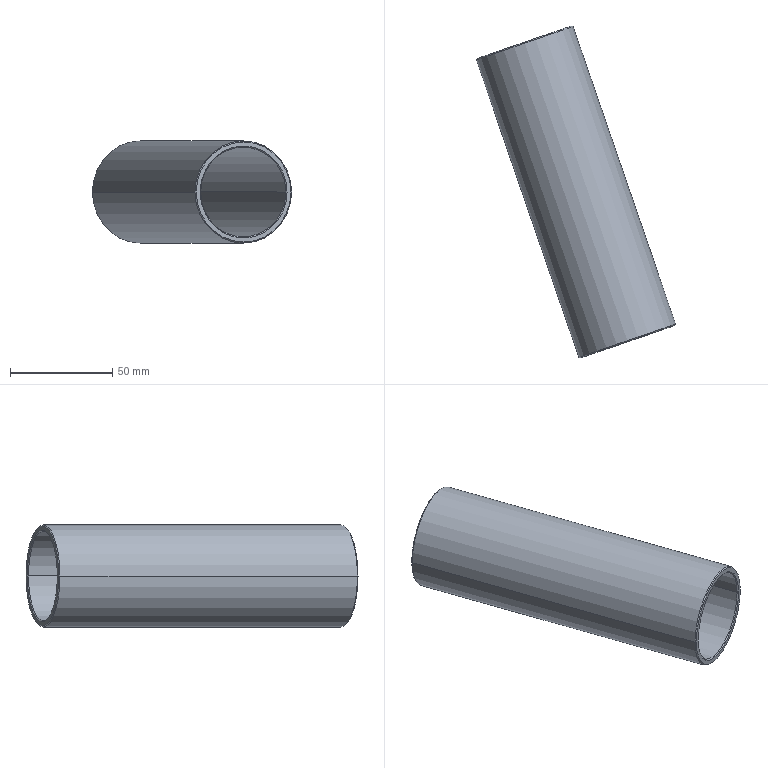Part | STEP file | PRT0001_68_1 | 1 solid | 14 faces | box 97.464 x 162.507 x 50 mm | volume 68590 mm3 | cone 8 | cylinder 4 | plane 2 | commonest cylinder face diameters 44 x2 50 x2
STEP:
#1=CARTESIAN_POINT('',(0.,0.,0.));
#2=DIRECTION('',(0.,0.,1.));
#3=DIRECTION('',(1.,0.,0.));
#4=AXIS2_PLACEMENT_3D('',#1,#2,#3);
#5=CARTESIAN_POINT('',(2166.559,1217.903,0.));
#6=VERTEX_POINT('',#5);
#7=CARTESIAN_POINT('',(2145.761,1210.732,22.));
#8=VERTEX_POINT('',#7);
#9=CARTESIAN_POINT('',(2145.761,1210.732,0.));
#10=DIRECTION('',(0.3259,-0.9454,0.));
#11=DIRECTION('',(0.9454,0.3259,0.));
#12=AXIS2_PLACEMENT_3D('',#9,#10,#11);
#13=CIRCLE('',#12,22.);
#14=CARTESIAN_POINT('',(2145.842,1210.496,0.));
#15=DIRECTION('',(0.3259,-0.9454,0.));
#16=DIRECTION('',(0.,0.,-1.));
#17=AXIS2_PLACEMENT_3D('',#14,#15,#16);
#18=CONICAL_SURFACE('',#17,22.25,0.7854);
#19=CARTESIAN_POINT('',(1.571,-0.25));
#20=DIRECTION('',(1.,0.));
#21=VECTOR('',#20,1.);
#22=LINE('',#19,#21);
#23=(GEOMETRIC_REPRESENTATION_CONTEXT(2)PARAMETRIC_REPRESENTATION_CONTEXT()REPRESENTATION_CONTEXT('',''));
#24=DEFINITIONAL_REPRESENTATION('',(#22),#23);
#25=PCURVE('',#18,#24);
#26=CARTESIAN_POINT('',(2092.545,1365.083,0.));
#27=DIRECTION('',(0.3259,-0.9454,0.));
#28=DIRECTION('',(-0.9454,-0.3259,0.));
#29=AXIS2_PLACEMENT_3D('',#26,#27,#28);
#30=CYLINDRICAL_SURFACE('',#29,22.);
#31=CARTESIAN_POINT('',(3.142,163.267));
#32=DIRECTION('',(1.,0.));
#33=VECTOR('',#32,1.);
#34=LINE('',#31,#33);
#35=(GEOMETRIC_REPRESENTATION_CONTEXT(2)PARAMETRIC_REPRESENTATION_CONTEXT()REPRESENTATION_CONTEXT('',''));
#36=DEFINITIONAL_REPRESENTATION('',(#34),#35);
#37=PCURVE('',#30,#36);
#38=SURFACE_CURVE('',#13,(#25,#37),.PCURVE_S1.);
#39=EDGE_CURVE('',#6,#8,#38,.T.);
#40=ORIENTED_EDGE('',*,*,#39,.T.);
#41=CARTESIAN_POINT('',(2124.962,1203.562,0.));
#42=VERTEX_POINT('',#41);
#43=CARTESIAN_POINT('',(2145.761,1210.732,0.));
#44=DIRECTION('',(0.3259,-0.9454,0.));
#45=DIRECTION('',(0.,0.,1.));
#46=AXIS2_PLACEMENT_3D('',#43,#44,#45);
#47=CIRCLE('',#46,22.);
#48=CARTESIAN_POINT('',(3.142,-0.25));
#49=DIRECTION('',(1.,0.));
#50=VECTOR('',#49,1.);
#51=LINE('',#48,#50);
#52=(GEOMETRIC_REPRESENTATION_CONTEXT(2)PARAMETRIC_REPRESENTATION_CONTEXT()REPRESENTATION_CONTEXT('',''));
#53=DEFINITIONAL_REPRESENTATION('',(#51),#52);
#54=PCURVE('',#18,#53);
#55=CARTESIAN_POINT('',(4.712,163.267));
#56=DIRECTION('',(1.,0.));
#57=VECTOR('',#56,1.);
#58=LINE('',#55,#57);
#59=(GEOMETRIC_REPRESENTATION_CONTEXT(2)PARAMETRIC_REPRESENTATION_CONTEXT()REPRESENTATION_CONTEXT('',''));
#60=DEFINITIONAL_REPRESENTATION('',(#58),#59);
#61=PCURVE('',#30,#60);
#62=SURFACE_CURVE('',#47,(#54,#61),.PCURVE_S1.);
#63=EDGE_CURVE('',#8,#42,#62,.T.);
#64=ORIENTED_EDGE('',*,*,#63,.T.);
#65=CARTESIAN_POINT('',(2124.653,1202.926,0.));
#66=VERTEX_POINT('',#65);
#67=CARTESIAN_POINT('',(2124.653,1202.926,0.));
#68=DIRECTION('',(0.438,0.899,0.));
#69=VECTOR('',#68,1.);
#70=LINE('',#67,#69);
#71=CARTESIAN_POINT('',(4.712,0.25));
#72=DIRECTION('',(0.,-1.));
#73=VECTOR('',#72,1.);
#74=LINE('',#71,#73);
#75=(GEOMETRIC_REPRESENTATION_CONTEXT(2)PARAMETRIC_REPRESENTATION_CONTEXT()REPRESENTATION_CONTEXT('',''));
#76=DEFINITIONAL_REPRESENTATION('',(#74),#75);
#77=PCURVE('',#18,#76);
#78=CARTESIAN_POINT('',(2145.842,1210.496,0.));
#79=DIRECTION('',(0.3259,-0.9454,0.));
#80=DIRECTION('',(0.,0.,-1.));
#81=AXIS2_PLACEMENT_3D('',#78,#79,#80);
#82=CONICAL_SURFACE('',#81,22.25,0.7854);
#83=CARTESIAN_POINT('',(4.712,0.25));
#84=DIRECTION('',(0.,-1.));
#85=VECTOR('',#84,1.);
#86=LINE('',#83,#85);
#87=(GEOMETRIC_REPRESENTATION_CONTEXT(2)PARAMETRIC_REPRESENTATION_CONTEXT()REPRESENTATION_CONTEXT('',''));
#88=DEFINITIONAL_REPRESENTATION('',(#86),#87);
#89=PCURVE('',#82,#88);
#90=SURFACE_CURVE('',#70,(#77,#89),.PCURVE_S1.);
#91=EDGE_CURVE('',#66,#42,#90,.T.);
#92=ORIENTED_EDGE('',*,*,#91,.F.);
#93=CARTESIAN_POINT('',(2145.924,1210.26,22.5));
#94=VERTEX_POINT('',#93);
#95=CARTESIAN_POINT('',(2145.924,1210.26,0.));
#96=DIRECTION('',(0.3259,-0.9454,0.));
#97=DIRECTION('',(0.,0.,1.));
#98=AXIS2_PLACEMENT_3D('',#95,#96,#97);
#99=CIRCLE('',#98,22.5);
#100=CARTESIAN_POINT('',(3.142,0.25));
#101=DIRECTION('',(1.,0.));
#102=VECTOR('',#101,1.);
#103=LINE('',#100,#102);
#104=(GEOMETRIC_REPRESENTATION_CONTEXT(2)PARAMETRIC_REPRESENTATION_CONTEXT()REPRESENTATION_CONTEXT('',''));
#105=DEFINITIONAL_REPRESENTATION('',(#103),#104);
#106=PCURVE('',#18,#105);
#107=CARTESIAN_POINT('',(2145.924,1210.26,0.));
#108=DIRECTION('',(0.3259,-0.9454,0.));
#109=DIRECTION('',(-0.9454,-0.3259,0.));
#110=AXIS2_PLACEMENT_3D('',#107,#108,#109);
#111=PLANE('',#110);
#112=CARTESIAN_POINT('',(-0.000000001,0.));
#113=DIRECTION('',(0.,-1.));
#114=AXIS2_PLACEMENT_2D('',#112,#113);
#115=CIRCLE('',#114,22.5);
#116=(GEOMETRIC_REPRESENTATION_CONTEXT(2)PARAMETRIC_REPRESENTATION_CONTEXT()REPRESENTATION_CONTEXT('',''));
#117=DEFINITIONAL_REPRESENTATION('',(#115),#116);
#118=PCURVE('',#111,#117);
#119=SURFACE_CURVE('',#99,(#106,#118),.PCURVE_S1.);
#120=EDGE_CURVE('',#94,#66,#119,.T.);
#121=ORIENTED_EDGE('',*,*,#120,.F.);
#122=CARTESIAN_POINT('',(2167.195,1217.593,0.));
#123=VERTEX_POINT('',#122);
#124=CARTESIAN_POINT('',(2145.924,1210.26,0.));
#125=DIRECTION('',(0.3259,-0.9454,0.));
#126=DIRECTION('',(0.9454,0.3259,0.));
#127=AXIS2_PLACEMENT_3D('',#124,#125,#126);
#128=CIRCLE('',#127,22.5);
#129=CARTESIAN_POINT('',(1.571,0.25));
#130=DIRECTION('',(1.,0.));
#131=VECTOR('',#130,1.);
#132=LINE('',#129,#131);
#133=(GEOMETRIC_REPRESENTATION_CONTEXT(2)PARAMETRIC_REPRESENTATION_CONTEXT()REPRESENTATION_CONTEXT('',''));
#134=DEFINITIONAL_REPRESENTATION('',(#132),#133);
#135=PCURVE('',#18,#134);
#136=CARTESIAN_POINT('',(-0.000000001,0.));
#137=DIRECTION('',(-1.,0.));
#138=AXIS2_PLACEMENT_2D('',#136,#137);
#139=CIRCLE('',#138,22.5);
#140=(GEOMETRIC_REPRESENTATION_CONTEXT(2)PARAMETRIC_REPRESENTATION_CONTEXT()REPRESENTATION_CONTEXT('',''));
#141=DEFINITIONAL_REPRESENTATION('',(#139),#140);
#142=PCURVE('',#111,#141);
#143=SURFACE_CURVE('',#128,(#135,#142),.PCURVE_S1.);
#144=EDGE_CURVE('',#123,#94,#143,.T.);
#145=ORIENTED_EDGE('',*,*,#144,.F.);
#146=CARTESIAN_POINT('',(2167.195,1217.593,0.));
#147=DIRECTION('',(-0.899,0.438,0.));
#148=VECTOR('',#147,1.);
#149=LINE('',#146,#148);
#150=CARTESIAN_POINT('',(1.571,0.25));
#151=DIRECTION('',(0.,-1.));
#152=VECTOR('',#151,1.);
#153=LINE('',#150,#152);
#154=(GEOMETRIC_REPRESENTATION_CONTEXT(2)PARAMETRIC_REPRESENTATION_CONTEXT()REPRESENTATION_CONTEXT('',''));
#155=DEFINITIONAL_REPRESENTATION('',(#153),#154);
#156=PCURVE('',#18,#155);
#157=CARTESIAN_POINT('',(7.854,0.25));
#158=DIRECTION('',(0.,-1.));
#159=VECTOR('',#158,1.);
#160=LINE('',#157,#159);
#161=(GEOMETRIC_REPRESENTATION_CONTEXT(2)PARAMETRIC_REPRESENTATION_CONTEXT()REPRESENTATION_CONTEXT('',''));
#162=DEFINITIONAL_REPRESENTATION('',(#160),#161);
#163=PCURVE('',#82,#162);
#164=SURFACE_CURVE('',#149,(#156,#163),.PCURVE_S1.);
#165=EDGE_CURVE('',#123,#6,#164,.T.);
#166=ORIENTED_EDGE('',*,*,#165,.T.);
#167=EDGE_LOOP('',(#40,#64,#92,#121,#145,#166));
#168=FACE_BOUND('',#167,.F.);
#169=ADVANCED_FACE('',(#168),#18,.F.);
#170=CARTESIAN_POINT('',(2095.566,1356.322,22.));
#171=VERTEX_POINT('',#170);
#172=CARTESIAN_POINT('',(2116.364,1363.493,0.));
#173=VERTEX_POINT('',#172);
#174=CARTESIAN_POINT('',(2095.566,1356.322,0.));
#175=DIRECTION('',(-0.3259,0.9454,0.));
#176=DIRECTION('',(0.,0.,1.));
#177=AXIS2_PLACEMENT_3D('',#174,#175,#176);
#178=CIRCLE('',#177,22.);
#179=CARTESIAN_POINT('',(4.712,9.267));
#180=DIRECTION('',(-1.,0.));
#181=VECTOR('',#180,1.);
#182=LINE('',#179,#181);
#183=(GEOMETRIC_REPRESENTATION_CONTEXT(2)PARAMETRIC_REPRESENTATION_CONTEXT()REPRESENTATION_CONTEXT('',''));
#184=DEFINITIONAL_REPRESENTATION('',(#182),#183);
#185=PCURVE('',#30,#184);
#186=CARTESIAN_POINT('',(2095.484,1356.559,0.));
#187=DIRECTION('',(-0.3259,0.9454,0.));
#188=DIRECTION('',(0.,0.,-1.));
#189=AXIS2_PLACEMENT_3D('',#186,#187,#188);
#190=CONICAL_SURFACE('',#189,22.25,0.7854);
#191=CARTESIAN_POINT('',(3.142,-0.25));
#192=DIRECTION('',(1.,0.));
#193=VECTOR('',#192,1.);
#194=LINE('',#191,#193);
#195=(GEOMETRIC_REPRESENTATION_CONTEXT(2)PARAMETRIC_REPRESENTATION_CONTEXT()REPRESENTATION_CONTEXT('',''));
#196=DEFINITIONAL_REPRESENTATION('',(#194),#195);
#197=PCURVE('',#190,#196);
#198=SURFACE_CURVE('',#178,(#185,#197),.PCURVE_S1.);
#199=EDGE_CURVE('',#171,#173,#198,.T.);
#200=ORIENTED_EDGE('',*,*,#199,.F.);
#201=CARTESIAN_POINT('',(2074.767,1349.152,0.));
#202=VERTEX_POINT('',#201);
#203=CARTESIAN_POINT('',(2095.566,1356.322,0.));
#204=DIRECTION('',(-0.3259,0.9454,0.));
#205=DIRECTION('',(-0.9454,-0.3259,0.));
#206=AXIS2_PLACEMENT_3D('',#203,#204,#205);
#207=CIRCLE('',#206,22.);
#208=CARTESIAN_POINT('',(6.283,9.267));
#209=DIRECTION('',(-1.,0.));
#210=VECTOR('',#209,1.);
#211=LINE('',#208,#210);
#212=(GEOMETRIC_REPRESENTATION_CONTEXT(2)PARAMETRIC_REPRESENTATION_CONTEXT()REPRESENTATION_CONTEXT('',''));
#213=DEFINITIONAL_REPRESENTATION('',(#211),#212);
#214=PCURVE('',#30,#213);
#215=CARTESIAN_POINT('',(1.571,-0.25));
#216=DIRECTION('',(1.,0.));
#217=VECTOR('',#216,1.);
#218=LINE('',#215,#217);
#219=(GEOMETRIC_REPRESENTATION_CONTEXT(2)PARAMETRIC_REPRESENTATION_CONTEXT()REPRESENTATION_CONTEXT('',''));
#220=DEFINITIONAL_REPRESENTATION('',(#218),#219);
#221=PCURVE('',#190,#220);
#222=SURFACE_CURVE('',#207,(#214,#221),.PCURVE_S1.);
#223=EDGE_CURVE('',#202,#171,#222,.T.);
#224=ORIENTED_EDGE('',*,*,#223,.F.);
#225=CARTESIAN_POINT('',(2074.767,1349.152,0.));
#226=DIRECTION('',(0.3259,-0.9454,0.));
#227=VECTOR('',#226,1.);
#228=LINE('',#225,#227);
#229=CARTESIAN_POINT('',(6.283,9.267));
#230=DIRECTION('',(0.,1.));
#231=VECTOR('',#230,1.);
#232=LINE('',#229,#231);
#233=(GEOMETRIC_REPRESENTATION_CONTEXT(2)PARAMETRIC_REPRESENTATION_CONTEXT()REPRESENTATION_CONTEXT('',''));
#234=DEFINITIONAL_REPRESENTATION('',(#232),#233);
#235=PCURVE('',#30,#234);
#236=CARTESIAN_POINT('',(2092.545,1365.083,0.));
#237=DIRECTION('',(0.3259,-0.9454,0.));
#238=DIRECTION('',(-0.9454,-0.3259,0.));
#239=AXIS2_PLACEMENT_3D('',#236,#237,#238);
#240=CYLINDRICAL_SURFACE('',#239,22.);
#241=CARTESIAN_POINT('',(0.,9.267));
#242=DIRECTION('',(0.,1.));
#243=VECTOR('',#242,1.);
#244=LINE('',#241,#243);
#245=(GEOMETRIC_REPRESENTATION_CONTEXT(2)PARAMETRIC_REPRESENTATION_CONTEXT()REPRESENTATION_CONTEXT('',''));
#246=DEFINITIONAL_REPRESENTATION('',(#244),#245);
#247=PCURVE('',#240,#246);
#248=SURFACE_CURVE('',#228,(#235,#247),.PCURVE_S1.);
#249=EDGE_CURVE('',#202,#42,#248,.T.);
#250=ORIENTED_EDGE('',*,*,#249,.T.);
#251=ORIENTED_EDGE('',*,*,#63,.F.);
#252=ORIENTED_EDGE('',*,*,#39,.F.);
#253=CARTESIAN_POINT('',(2116.364,1363.493,0.));
#254=DIRECTION('',(0.3259,-0.9454,0.));
#255=VECTOR('',#254,1.);
#256=LINE('',#253,#255);
#257=CARTESIAN_POINT('',(3.142,9.267));
#258=DIRECTION('',(0.,1.));
#259=VECTOR('',#258,1.);
#260=LINE('',#257,#259);
#261=(GEOMETRIC_REPRESENTATION_CONTEXT(2)PARAMETRIC_REPRESENTATION_CONTEXT()REPRESENTATION_CONTEXT('',''));
#262=DEFINITIONAL_REPRESENTATION('',(#260),#261);
#263=PCURVE('',#30,#262);
#264=CARTESIAN_POINT('',(3.142,9.267));
#265=DIRECTION('',(0.,1.));
#266=VECTOR('',#265,1.);
#267=LINE('',#264,#266);
#268=(GEOMETRIC_REPRESENTATION_CONTEXT(2)PARAMETRIC_REPRESENTATION_CONTEXT()REPRESENTATION_CONTEXT('',''));
#269=DEFINITIONAL_REPRESENTATION('',(#267),#268);
#270=PCURVE('',#240,#269);
#271=SURFACE_CURVE('',#256,(#263,#270),.PCURVE_S1.);
#272=EDGE_CURVE('',#173,#6,#271,.T.);
#273=ORIENTED_EDGE('',*,*,#272,.F.);
#274=EDGE_LOOP('',(#200,#224,#250,#251,#252,#273));
#275=FACE_BOUND('',#274,.F.);
#276=ADVANCED_FACE('',(#275),#30,.F.);
#277=CARTESIAN_POINT('',(2095.403,1356.795,22.5));
#278=VERTEX_POINT('',#277);
#279=CARTESIAN_POINT('',(2116.674,1364.129,0.));
#280=VERTEX_POINT('',#279);
#281=CARTESIAN_POINT('',(2095.403,1356.795,0.));
#282=DIRECTION('',(-0.3259,0.9454,0.));
#283=DIRECTION('',(0.,0.,1.));
#284=AXIS2_PLACEMENT_3D('',#281,#282,#283);
#285=CIRCLE('',#284,22.5);
#286=CARTESIAN_POINT('',(3.142,0.25));
#287=DIRECTION('',(1.,0.));
#288=VECTOR('',#287,1.);
#289=LINE('',#286,#288);
#290=(GEOMETRIC_REPRESENTATION_CONTEXT(2)PARAMETRIC_REPRESENTATION_CONTEXT()REPRESENTATION_CONTEXT('',''));
#291=DEFINITIONAL_REPRESENTATION('',(#289),#290);
#292=PCURVE('',#190,#291);
#293=CARTESIAN_POINT('',(2095.403,1356.795,0.));
#294=DIRECTION('',(0.3259,-0.9454,0.));
#295=DIRECTION('',(-0.9454,-0.3259,0.));
#296=AXIS2_PLACEMENT_3D('',#293,#294,#295);
#297=PLANE('',#296);
#298=CARTESIAN_POINT('',(0.,-22.5));
#299=CARTESIAN_POINT('',(-38.971,-22.5));
#300=CARTESIAN_POINT('',(-19.485,11.25));
#301=CARTESIAN_POINT('',(0.,45.));
#302=CARTESIAN_POINT('',(19.485,11.25));
#303=CARTESIAN_POINT('',(38.971,-22.5));
#304=CARTESIAN_POINT('',(0.,-22.5));
#305=(BOUNDED_CURVE()B_SPLINE_CURVE(2,(#298,#299,#300,#301,#302,#303,#304),.UNSPECIFIED.,.T.,.F.)B_SPLINE_CURVE_WITH_KNOTS((1,2,2,2,2,1),(-2.094,0.,2.094,4.189,6.283,8.378),.UNSPECIFIED.)CURVE()GEOMETRIC_REPRESENTATION_ITEM()RATIONAL_B_SPLINE_CURVE((1.,0.5,1.,0.5,1.,0.5,1.))REPRESENTATION_ITEM(''));
#306=(GEOMETRIC_REPRESENTATION_CONTEXT(2)PARAMETRIC_REPRESENTATION_CONTEXT()REPRESENTATION_CONTEXT('',''));
#307=DEFINITIONAL_REPRESENTATION('',(#305),#306);
#308=PCURVE('',#297,#307);
#309=SURFACE_CURVE('',#285,(#292,#308),.PCURVE_S1.);
#310=EDGE_CURVE('',#278,#280,#309,.T.);
#311=ORIENTED_EDGE('',*,*,#310,.F.);
#312=CARTESIAN_POINT('',(2074.132,1349.461,0.));
#313=VERTEX_POINT('',#312);
#314=CARTESIAN_POINT('',(2095.403,1356.795,0.));
#315=DIRECTION('',(-0.3259,0.9454,0.));
#316=DIRECTION('',(-0.9454,-0.3259,0.));
#317=AXIS2_PLACEMENT_3D('',#314,#315,#316);
#318=CIRCLE('',#317,22.5);
#319=CARTESIAN_POINT('',(1.571,0.25));
#320=DIRECTION('',(1.,0.));
#321=VECTOR('',#320,1.);
#322=LINE('',#319,#321);
#323=(GEOMETRIC_REPRESENTATION_CONTEXT(2)PARAMETRIC_REPRESENTATION_CONTEXT()REPRESENTATION_CONTEXT('',''));
#324=DEFINITIONAL_REPRESENTATION('',(#322),#323);
#325=PCURVE('',#190,#324);
#326=CARTESIAN_POINT('',(22.5,0.));
#327=CARTESIAN_POINT('',(22.5,-38.971));
#328=CARTESIAN_POINT('',(-11.25,-19.485));
#329=CARTESIAN_POINT('',(-45.,0.));
#330=CARTESIAN_POINT('',(-11.25,19.485));
#331=CARTESIAN_POINT('',(22.5,38.971));
#332=CARTESIAN_POINT('',(22.5,0.));
#333=(BOUNDED_CURVE()B_SPLINE_CURVE(2,(#326,#327,#328,#329,#330,#331,#332),.UNSPECIFIED.,.T.,.F.)B_SPLINE_CURVE_WITH_KNOTS((1,2,2,2,2,1),(-2.094,0.,2.094,4.189,6.283,8.378),.UNSPECIFIED.)CURVE()GEOMETRIC_REPRESENTATION_ITEM()RATIONAL_B_SPLINE_CURVE((1.,0.5,1.,0.5,1.,0.5,1.))REPRESENTATION_ITEM(''));
#334=(GEOMETRIC_REPRESENTATION_CONTEXT(2)PARAMETRIC_REPRESENTATION_CONTEXT()REPRESENTATION_CONTEXT('',''));
#335=DEFINITIONAL_REPRESENTATION('',(#333),#334);
#336=PCURVE('',#297,#335);
#337=SURFACE_CURVE('',#318,(#325,#336),.PCURVE_S1.);
#338=EDGE_CURVE('',#313,#278,#337,.T.);
#339=ORIENTED_EDGE('',*,*,#338,.F.);
#340=CARTESIAN_POINT('',(2074.767,1349.152,0.));
#341=DIRECTION('',(-0.899,0.438,0.));
#342=VECTOR('',#341,1.);
#343=LINE('',#340,#342);
#344=CARTESIAN_POINT('',(1.571,-0.25));
#345=DIRECTION('',(0.,1.));
#346=VECTOR('',#345,1.);
#347=LINE('',#344,#346);
#348=(GEOMETRIC_REPRESENTATION_CONTEXT(2)PARAMETRIC_REPRESENTATION_CONTEXT()REPRESENTATION_CONTEXT('',''));
#349=DEFINITIONAL_REPRESENTATION('',(#347),#348);
#350=PCURVE('',#190,#349);
#351=CARTESIAN_POINT('',(2095.484,1356.559,0.));
#352=DIRECTION('',(-0.3259,0.9454,0.));
#353=DIRECTION('',(0.,0.,-1.));
#354=AXIS2_PLACEMENT_3D('',#351,#352,#353);
#355=CONICAL_SURFACE('',#354,22.25,0.7854);
#356=CARTESIAN_POINT('',(1.571,-0.25));
#357=DIRECTION('',(0.,1.));
#358=VECTOR('',#357,1.);
#359=LINE('',#356,#358);
#360=(GEOMETRIC_REPRESENTATION_CONTEXT(2)PARAMETRIC_REPRESENTATION_CONTEXT()REPRESENTATION_CONTEXT('',''));
#361=DEFINITIONAL_REPRESENTATION('',(#359),#360);
#362=PCURVE('',#355,#361);
#363=SURFACE_CURVE('',#343,(#350,#362),.PCURVE_S1.);
#364=EDGE_CURVE('',#202,#313,#363,.T.);
#365=ORIENTED_EDGE('',*,*,#364,.F.);
#366=ORIENTED_EDGE('',*,*,#223,.T.);
#367=ORIENTED_EDGE('',*,*,#199,.T.);
#368=CARTESIAN_POINT('',(2116.364,1363.493,0.));
#369=DIRECTION('',(0.438,0.899,0.));
#370=VECTOR('',#369,1.);
#371=LINE('',#368,#370);
#372=CARTESIAN_POINT('',(4.712,-0.25));
#373=DIRECTION('',(0.,1.));
#374=VECTOR('',#373,1.);
#375=LINE('',#372,#374);
#376=(GEOMETRIC_REPRESENTATION_CONTEXT(2)PARAMETRIC_REPRESENTATION_CONTEXT()REPRESENTATION_CONTEXT('',''));
#377=DEFINITIONAL_REPRESENTATION('',(#375),#376);
#378=PCURVE('',#190,#377);
#379=CARTESIAN_POINT('',(-1.571,-0.25));
#380=DIRECTION('',(0.,1.));
#381=VECTOR('',#380,1.);
#382=LINE('',#379,#381);
#383=(GEOMETRIC_REPRESENTATION_CONTEXT(2)PARAMETRIC_REPRESENTATION_CONTEXT()REPRESENTATION_CONTEXT('',''));
#384=DEFINITIONAL_REPRESENTATION('',(#382),#383);
#385=PCURVE('',#355,#384);
#386=SURFACE_CURVE('',#371,(#378,#385),.PCURVE_S1.);
#387=EDGE_CURVE('',#173,#280,#386,.T.);
#388=ORIENTED_EDGE('',*,*,#387,.T.);
#389=EDGE_LOOP('',(#311,#339,#365,#366,#367,#388));
#390=FACE_BOUND('',#389,.F.);
#391=ADVANCED_FACE('',(#390),#190,.F.);
#392=CARTESIAN_POINT('',(2072.241,1348.809,0.));
#393=VERTEX_POINT('',#392);
#394=CARTESIAN_POINT('',(2095.403,1356.795,-24.5));
#395=VERTEX_POINT('',#394);
#396=CARTESIAN_POINT('',(2095.403,1356.795,0.));
#397=DIRECTION('',(0.3259,-0.9454,0.));
#398=DIRECTION('',(-0.9454,-0.3259,0.));
#399=AXIS2_PLACEMENT_3D('',#396,#397,#398);
#400=CIRCLE('',#399,24.5);
#401=CARTESIAN_POINT('',(0.,0.));
#402=DIRECTION('',(1.,0.));
#403=AXIS2_PLACEMENT_2D('',#401,#402);
#404=CIRCLE('',#403,24.5);
#405=(GEOMETRIC_REPRESENTATION_CONTEXT(2)PARAMETRIC_REPRESENTATION_CONTEXT()REPRESENTATION_CONTEXT('',''));
#406=DEFINITIONAL_REPRESENTATION('',(#404),#405);
#407=PCURVE('',#297,#406);
#408=CARTESIAN_POINT('',(2095.484,1356.559,0.));
#409=DIRECTION('',(0.3259,-0.9454,0.));
#410=DIRECTION('',(0.,0.,-1.));
#411=AXIS2_PLACEMENT_3D('',#408,#409,#410);
#412=CONICAL_SURFACE('',#411,24.75,0.7854);
#413=CARTESIAN_POINT('',(-1.571,-0.25));
#414=DIRECTION('',(1.,0.));
#415=VECTOR('',#414,1.);
#416=LINE('',#413,#415);
#417=(GEOMETRIC_REPRESENTATION_CONTEXT(2)PARAMETRIC_REPRESENTATION_CONTEXT()REPRESENTATION_CONTEXT('',''));
#418=DEFINITIONAL_REPRESENTATION('',(#416),#417);
#419=PCURVE('',#412,#418);
#420=SURFACE_CURVE('',#400,(#407,#419),.PCURVE_S1.);
#421=EDGE_CURVE('',#393,#395,#420,.T.);
#422=ORIENTED_EDGE('',*,*,#421,.T.);
#423=CARTESIAN_POINT('',(2118.565,1364.781,0.));
#424=VERTEX_POINT('',#423);
#425=CARTESIAN_POINT('',(2095.403,1356.795,0.));
#426=DIRECTION('',(0.3259,-0.9454,0.));
#427=DIRECTION('',(0.,0.,-1.));
#428=AXIS2_PLACEMENT_3D('',#425,#426,#427);
#429=CIRCLE('',#428,24.5);
#430=CARTESIAN_POINT('',(0.,0.));
#431=DIRECTION('',(0.,1.));
#432=AXIS2_PLACEMENT_2D('',#430,#431);
#433=CIRCLE('',#432,24.5);
#434=(GEOMETRIC_REPRESENTATION_CONTEXT(2)PARAMETRIC_REPRESENTATION_CONTEXT()REPRESENTATION_CONTEXT('',''));
#435=DEFINITIONAL_REPRESENTATION('',(#433),#434);
#436=PCURVE('',#297,#435);
#437=CARTESIAN_POINT('',(0.,-0.25));
#438=DIRECTION('',(1.,0.));
#439=VECTOR('',#438,1.);
#440=LINE('',#437,#439);
#441=(GEOMETRIC_REPRESENTATION_CONTEXT(2)PARAMETRIC_REPRESENTATION_CONTEXT()REPRESENTATION_CONTEXT('',''));
#442=DEFINITIONAL_REPRESENTATION('',(#440),#441);
#443=PCURVE('',#412,#442);
#444=SURFACE_CURVE('',#429,(#436,#443),.PCURVE_S1.);
#445=EDGE_CURVE('',#395,#424,#444,.T.);
#446=ORIENTED_EDGE('',*,*,#445,.T.);
#447=CARTESIAN_POINT('',(2095.403,1356.795,24.5));
#448=VERTEX_POINT('',#447);
#449=CARTESIAN_POINT('',(2095.403,1356.795,0.));
#450=DIRECTION('',(0.3259,-0.9454,0.));
#451=DIRECTION('',(0.9454,0.3259,0.));
#452=AXIS2_PLACEMENT_3D('',#449,#450,#451);
#453=CIRCLE('',#452,24.5);
#454=CARTESIAN_POINT('',(0.,0.));
#455=DIRECTION('',(-1.,0.));
#456=AXIS2_PLACEMENT_2D('',#454,#455);
#457=CIRCLE('',#456,24.5);
#458=(GEOMETRIC_REPRESENTATION_CONTEXT(2)PARAMETRIC_REPRESENTATION_CONTEXT()REPRESENTATION_CONTEXT('',''));
#459=DEFINITIONAL_REPRESENTATION('',(#457),#458);
#460=PCURVE('',#297,#459);
#461=CARTESIAN_POINT('',(2095.484,1356.559,0.));
#462=DIRECTION('',(0.3259,-0.9454,0.));
#463=DIRECTION('',(0.,0.,-1.));
#464=AXIS2_PLACEMENT_3D('',#461,#462,#463);
#465=CONICAL_SURFACE('',#464,24.75,0.7854);
#466=CARTESIAN_POINT('',(1.571,-0.25));
#467=DIRECTION('',(1.,0.));
#468=VECTOR('',#467,1.);
#469=LINE('',#466,#468);
#470=(GEOMETRIC_REPRESENTATION_CONTEXT(2)PARAMETRIC_REPRESENTATION_CONTEXT()REPRESENTATION_CONTEXT('',''));
#471=DEFINITIONAL_REPRESENTATION('',(#469),#470);
#472=PCURVE('',#465,#471);
#473=SURFACE_CURVE('',#453,(#460,#472),.PCURVE_S1.);
#474=EDGE_CURVE('',#424,#448,#473,.T.);
#475=ORIENTED_EDGE('',*,*,#474,.T.);
#476=CARTESIAN_POINT('',(2095.403,1356.795,0.));
#477=DIRECTION('',(0.3259,-0.9454,0.));
#478=DIRECTION('',(0.,0.,1.));
#479=AXIS2_PLACEMENT_3D('',#476,#477,#478);
#480=CIRCLE('',#479,24.5);
#481=CARTESIAN_POINT('',(0.,0.));
#482=DIRECTION('',(0.,-1.));
#483=AXIS2_PLACEMENT_2D('',#481,#482);
#484=CIRCLE('',#483,24.5);
#485=(GEOMETRIC_REPRESENTATION_CONTEXT(2)PARAMETRIC_REPRESENTATION_CONTEXT()REPRESENTATION_CONTEXT('',''));
#486=DEFINITIONAL_REPRESENTATION('',(#484),#485);
#487=PCURVE('',#297,#486);
#488=CARTESIAN_POINT('',(3.142,-0.25));
#489=DIRECTION('',(1.,0.));
#490=VECTOR('',#489,1.);
#491=LINE('',#488,#490);
#492=(GEOMETRIC_REPRESENTATION_CONTEXT(2)PARAMETRIC_REPRESENTATION_CONTEXT()REPRESENTATION_CONTEXT('',''));
#493=DEFINITIONAL_REPRESENTATION('',(#491),#492);
#494=PCURVE('',#465,#493);
#495=SURFACE_CURVE('',#480,(#487,#494),.PCURVE_S1.);
#496=EDGE_CURVE('',#448,#393,#495,.T.);
#497=ORIENTED_EDGE('',*,*,#496,.T.);
#498=EDGE_LOOP('',(#422,#446,#475,#497));
#499=FACE_BOUND('',#498,.F.);
#500=CARTESIAN_POINT('',(2095.403,1356.795,-22.5));
#501=VERTEX_POINT('',#500);
#502=CARTESIAN_POINT('',(2095.403,1356.795,0.));
#503=DIRECTION('',(-0.3259,0.9454,0.));
#504=DIRECTION('',(0.9454,0.3259,0.));
#505=AXIS2_PLACEMENT_3D('',#502,#503,#504);
#506=CIRCLE('',#505,22.5);
#507=CARTESIAN_POINT('',(-22.5,0.));
#508=CARTESIAN_POINT('',(-22.5,38.971));
#509=CARTESIAN_POINT('',(11.25,19.485));
#510=CARTESIAN_POINT('',(45.,0.));
#511=CARTESIAN_POINT('',(11.25,-19.485));
#512=CARTESIAN_POINT('',(-22.5,-38.971));
#513=CARTESIAN_POINT('',(-22.5,0.));
#514=(BOUNDED_CURVE()B_SPLINE_CURVE(2,(#507,#508,#509,#510,#511,#512,#513),.UNSPECIFIED.,.T.,.F.)B_SPLINE_CURVE_WITH_KNOTS((1,2,2,2,2,1),(-2.094,0.,2.094,4.189,6.283,8.378),.UNSPECIFIED.)CURVE()GEOMETRIC_REPRESENTATION_ITEM()RATIONAL_B_SPLINE_CURVE((1.,0.5,1.,0.5,1.,0.5,1.))REPRESENTATION_ITEM(''));
#515=(GEOMETRIC_REPRESENTATION_CONTEXT(2)PARAMETRIC_REPRESENTATION_CONTEXT()REPRESENTATION_CONTEXT('',''));
#516=DEFINITIONAL_REPRESENTATION('',(#514),#515);
#517=PCURVE('',#297,#516);
#518=CARTESIAN_POINT('',(-1.571,0.25));
#519=DIRECTION('',(1.,0.));
#520=VECTOR('',#519,1.);
#521=LINE('',#518,#520);
#522=(GEOMETRIC_REPRESENTATION_CONTEXT(2)PARAMETRIC_REPRESENTATION_CONTEXT()REPRESENTATION_CONTEXT('',''));
#523=DEFINITIONAL_REPRESENTATION('',(#521),#522);
#524=PCURVE('',#355,#523);
#525=SURFACE_CURVE('',#506,(#517,#524),.PCURVE_S1.);
#526=EDGE_CURVE('',#280,#501,#525,.T.);
#527=ORIENTED_EDGE('',*,*,#526,.T.);
#528=CARTESIAN_POINT('',(2095.403,1356.795,0.));
#529=DIRECTION('',(-0.3259,0.9454,0.));
#530=DIRECTION('',(0.,0.,-1.));
#531=AXIS2_PLACEMENT_3D('',#528,#529,#530);
#532=CIRCLE('',#531,22.5);
#533=CARTESIAN_POINT('',(0.,22.5));
#534=CARTESIAN_POINT('',(38.971,22.5));
#535=CARTESIAN_POINT('',(19.485,-11.25));
#536=CARTESIAN_POINT('',(0.,-45.));
#537=CARTESIAN_POINT('',(-19.485,-11.25));
#538=CARTESIAN_POINT('',(-38.971,22.5));
#539=CARTESIAN_POINT('',(0.,22.5));
#540=(BOUNDED_CURVE()B_SPLINE_CURVE(2,(#533,#534,#535,#536,#537,#538,#539),.UNSPECIFIED.,.T.,.F.)B_SPLINE_CURVE_WITH_KNOTS((1,2,2,2,2,1),(-2.094,0.,2.094,4.189,6.283,8.378),.UNSPECIFIED.)CURVE()GEOMETRIC_REPRESENTATION_ITEM()RATIONAL_B_SPLINE_CURVE((1.,0.5,1.,0.5,1.,0.5,1.))REPRESENTATION_ITEM(''));
#541=(GEOMETRIC_REPRESENTATION_CONTEXT(2)PARAMETRIC_REPRESENTATION_CONTEXT()REPRESENTATION_CONTEXT('',''));
#542=DEFINITIONAL_REPRESENTATION('',(#540),#541);
#543=PCURVE('',#297,#542);
#544=CARTESIAN_POINT('',(0.,0.25));
#545=DIRECTION('',(1.,0.));
#546=VECTOR('',#545,1.);
#547=LINE('',#544,#546);
#548=(GEOMETRIC_REPRESENTATION_CONTEXT(2)PARAMETRIC_REPRESENTATION_CONTEXT()REPRESENTATION_CONTEXT('',''));
#549=DEFINITIONAL_REPRESENTATION('',(#547),#548);
#550=PCURVE('',#355,#549);
#551=SURFACE_CURVE('',#532,(#543,#550),.PCURVE_S1.);
#552=EDGE_CURVE('',#501,#313,#551,.T.);
#553=ORIENTED_EDGE('',*,*,#552,.T.);
#554=ORIENTED_EDGE('',*,*,#338,.T.);
#555=ORIENTED_EDGE('',*,*,#310,.T.);
#556=EDGE_LOOP('',(#527,#553,#554,#555));
#557=FACE_BOUND('',#556,.F.);
#558=ADVANCED_FACE('',(#499,#557),#297,.F.);
#559=CARTESIAN_POINT('',(2071.931,1348.174,0.));
#560=VERTEX_POINT('',#559);
#561=CARTESIAN_POINT('',(2072.241,1348.809,0.));
#562=DIRECTION('',(-0.438,-0.899,0.));
#563=VECTOR('',#562,1.);
#564=LINE('',#561,#563);
#565=CARTESIAN_POINT('',(-1.571,-0.25));
#566=DIRECTION('',(0.,1.));
#567=VECTOR('',#566,1.);
#568=LINE('',#565,#567);
#569=(GEOMETRIC_REPRESENTATION_CONTEXT(2)PARAMETRIC_REPRESENTATION_CONTEXT()REPRESENTATION_CONTEXT('',''));
#570=DEFINITIONAL_REPRESENTATION('',(#568),#569);
#571=PCURVE('',#412,#570);
#572=CARTESIAN_POINT('',(4.712,-0.25));
#573=DIRECTION('',(0.,1.));
#574=VECTOR('',#573,1.);
#575=LINE('',#572,#574);
#576=(GEOMETRIC_REPRESENTATION_CONTEXT(2)PARAMETRIC_REPRESENTATION_CONTEXT()REPRESENTATION_CONTEXT('',''));
#577=DEFINITIONAL_REPRESENTATION('',(#575),#576);
#578=PCURVE('',#465,#577);
#579=SURFACE_CURVE('',#564,(#571,#578),.PCURVE_S1.);
#580=EDGE_CURVE('',#393,#560,#579,.T.);
#581=ORIENTED_EDGE('',*,*,#580,.F.);
#582=ORIENTED_EDGE('',*,*,#421,.T.);
#583=ORIENTED_EDGE('',*,*,#445,.T.);
#584=CARTESIAN_POINT('',(2119.201,1364.471,0.));
#585=VERTEX_POINT('',#584);
#586=CARTESIAN_POINT('',(2118.565,1364.781,0.));
#587=DIRECTION('',(0.899,-0.438,0.));
#588=VECTOR('',#587,1.);
#589=LINE('',#586,#588);
#590=CARTESIAN_POINT('',(1.571,-0.25));
#591=DIRECTION('',(0.,1.));
#592=VECTOR('',#591,1.);
#593=LINE('',#590,#592);
#594=(GEOMETRIC_REPRESENTATION_CONTEXT(2)PARAMETRIC_REPRESENTATION_CONTEXT()REPRESENTATION_CONTEXT('',''));
#595=DEFINITIONAL_REPRESENTATION('',(#593),#594);
#596=PCURVE('',#412,#595);
#597=CARTESIAN_POINT('',(1.571,-0.25));
#598=DIRECTION('',(0.,1.));
#599=VECTOR('',#598,1.);
#600=LINE('',#597,#599);
#601=(GEOMETRIC_REPRESENTATION_CONTEXT(2)PARAMETRIC_REPRESENTATION_CONTEXT()REPRESENTATION_CONTEXT('',''));
#602=DEFINITIONAL_REPRESENTATION('',(#600),#601);
#603=PCURVE('',#465,#602);
#604=SURFACE_CURVE('',#589,(#596,#603),.PCURVE_S1.);
#605=EDGE_CURVE('',#424,#585,#604,.T.);
#606=ORIENTED_EDGE('',*,*,#605,.T.);
#607=CARTESIAN_POINT('',(2095.566,1356.322,-25.));
#608=VERTEX_POINT('',#607);
#609=CARTESIAN_POINT('',(2095.566,1356.322,0.));
#610=DIRECTION('',(0.3259,-0.9454,0.));
#611=DIRECTION('',(0.,0.,-1.));
#612=AXIS2_PLACEMENT_3D('',#609,#610,#611);
#613=CIRCLE('',#612,25.);
#614=CARTESIAN_POINT('',(0.,0.25));
#615=DIRECTION('',(1.,0.));
#616=VECTOR('',#615,1.);
#617=LINE('',#614,#616);
#618=(GEOMETRIC_REPRESENTATION_CONTEXT(2)PARAMETRIC_REPRESENTATION_CONTEXT()REPRESENTATION_CONTEXT('',''));
#619=DEFINITIONAL_REPRESENTATION('',(#617),#618);
#620=PCURVE('',#412,#619);
#621=CARTESIAN_POINT('',(2092.545,1365.083,0.));
#622=DIRECTION('',(0.3259,-0.9454,0.));
#623=DIRECTION('',(-0.9454,-0.3259,0.));
#624=AXIS2_PLACEMENT_3D('',#621,#622,#623);
#625=CYLINDRICAL_SURFACE('',#624,25.);
#626=CARTESIAN_POINT('',(1.571,9.267));
#627=DIRECTION('',(1.,0.));
#628=VECTOR('',#627,1.);
#629=LINE('',#626,#628);
#630=(GEOMETRIC_REPRESENTATION_CONTEXT(2)PARAMETRIC_REPRESENTATION_CONTEXT()REPRESENTATION_CONTEXT('',''));
#631=DEFINITIONAL_REPRESENTATION('',(#629),#630);
#632=PCURVE('',#625,#631);
#633=SURFACE_CURVE('',#613,(#620,#632),.PCURVE_S1.);
#634=EDGE_CURVE('',#608,#585,#633,.T.);
#635=ORIENTED_EDGE('',*,*,#634,.F.);
#636=CARTESIAN_POINT('',(2095.566,1356.322,0.));
#637=DIRECTION('',(0.3259,-0.9454,0.));
#638=DIRECTION('',(-0.9454,-0.3259,0.));
#639=AXIS2_PLACEMENT_3D('',#636,#637,#638);
#640=CIRCLE('',#639,25.);
#641=CARTESIAN_POINT('',(-1.571,0.25));
#642=DIRECTION('',(1.,0.));
#643=VECTOR('',#642,1.);
#644=LINE('',#641,#643);
#645=(GEOMETRIC_REPRESENTATION_CONTEXT(2)PARAMETRIC_REPRESENTATION_CONTEXT()REPRESENTATION_CONTEXT('',''));
#646=DEFINITIONAL_REPRESENTATION('',(#644),#645);
#647=PCURVE('',#412,#646);
#648=CARTESIAN_POINT('',(0.,9.267));
#649=DIRECTION('',(1.,0.));
#650=VECTOR('',#649,1.);
#651=LINE('',#648,#650);
#652=(GEOMETRIC_REPRESENTATION_CONTEXT(2)PARAMETRIC_REPRESENTATION_CONTEXT()REPRESENTATION_CONTEXT('',''));
#653=DEFINITIONAL_REPRESENTATION('',(#651),#652);
#654=PCURVE('',#625,#653);
#655=SURFACE_CURVE('',#640,(#647,#654),.PCURVE_S1.);
#656=EDGE_CURVE('',#560,#608,#655,.T.);
#657=ORIENTED_EDGE('',*,*,#656,.F.);
#658=EDGE_LOOP('',(#581,#582,#583,#606,#635,#657));
#659=FACE_BOUND('',#658,.T.);
#660=ADVANCED_FACE('',(#659),#412,.T.);
#661=CARTESIAN_POINT('',(2169.396,1218.881,0.));
#662=VERTEX_POINT('',#661);
#663=CARTESIAN_POINT('',(2169.396,1218.881,0.));
#664=DIRECTION('',(-0.3259,0.9454,0.));
#665=VECTOR('',#664,1.);
#666=LINE('',#663,#665);
#667=CARTESIAN_POINT('',(3.142,163.267));
#668=DIRECTION('',(0.,-1.));
#669=VECTOR('',#668,1.);
#670=LINE('',#667,#669);
#671=(GEOMETRIC_REPRESENTATION_CONTEXT(2)PARAMETRIC_REPRESENTATION_CONTEXT()REPRESENTATION_CONTEXT('',''));
#672=DEFINITIONAL_REPRESENTATION('',(#670),#671);
#673=PCURVE('',#625,#672);
#674=CARTESIAN_POINT('',(2092.545,1365.083,0.));
#675=DIRECTION('',(0.3259,-0.9454,0.));
#676=DIRECTION('',(-0.9454,-0.3259,0.));
#677=AXIS2_PLACEMENT_3D('',#674,#675,#676);
#678=CYLINDRICAL_SURFACE('',#677,25.);
#679=CARTESIAN_POINT('',(3.142,163.267));
#680=DIRECTION('',(0.,-1.));
#681=VECTOR('',#680,1.);
#682=LINE('',#679,#681);
#683=(GEOMETRIC_REPRESENTATION_CONTEXT(2)PARAMETRIC_REPRESENTATION_CONTEXT()REPRESENTATION_CONTEXT('',''));
#684=DEFINITIONAL_REPRESENTATION('',(#682),#683);
#685=PCURVE('',#678,#684);
#686=SURFACE_CURVE('',#666,(#673,#685),.PCURVE_S1.);
#687=EDGE_CURVE('',#662,#585,#686,.T.);
#688=ORIENTED_EDGE('',*,*,#687,.F.);
#689=CARTESIAN_POINT('',(2145.761,1210.732,-25.));
#690=VERTEX_POINT('',#689);
#691=CARTESIAN_POINT('',(2145.761,1210.732,0.));
#692=DIRECTION('',(-0.3259,0.9454,0.));
#693=DIRECTION('',(0.9454,0.3259,0.));
#694=AXIS2_PLACEMENT_3D('',#691,#692,#693);
#695=CIRCLE('',#694,25.);
#696=CARTESIAN_POINT('',(3.142,163.267));
#697=DIRECTION('',(-1.,0.));
#698=VECTOR('',#697,1.);
#699=LINE('',#696,#698);
#700=(GEOMETRIC_REPRESENTATION_CONTEXT(2)PARAMETRIC_REPRESENTATION_CONTEXT()REPRESENTATION_CONTEXT('',''));
#701=DEFINITIONAL_REPRESENTATION('',(#699),#700);
#702=PCURVE('',#625,#701);
#703=CARTESIAN_POINT('',(2145.842,1210.496,0.));
#704=DIRECTION('',(-0.3259,0.9454,0.));
#705=DIRECTION('',(0.,0.,-1.));
#706=AXIS2_PLACEMENT_3D('',#703,#704,#705);
#707=CONICAL_SURFACE('',#706,24.75,0.7854);
#708=CARTESIAN_POINT('',(-1.571,0.25));
#709=DIRECTION('',(1.,0.));
#710=VECTOR('',#709,1.);
#711=LINE('',#708,#710);
#712=(GEOMETRIC_REPRESENTATION_CONTEXT(2)PARAMETRIC_REPRESENTATION_CONTEXT()REPRESENTATION_CONTEXT('',''));
#713=DEFINITIONAL_REPRESENTATION('',(#711),#712);
#714=PCURVE('',#707,#713);
#715=SURFACE_CURVE('',#695,(#702,#714),.PCURVE_S1.);
#716=EDGE_CURVE('',#662,#690,#715,.T.);
#717=ORIENTED_EDGE('',*,*,#716,.T.);
#718=CARTESIAN_POINT('',(2122.126,1202.584,0.));
#719=VERTEX_POINT('',#718);
#720=CARTESIAN_POINT('',(2145.761,1210.732,0.));
#721=DIRECTION('',(-0.3259,0.9454,0.));
#722=DIRECTION('',(0.,0.,-1.));
#723=AXIS2_PLACEMENT_3D('',#720,#721,#722);
#724=CIRCLE('',#723,25.);
#725=CARTESIAN_POINT('',(1.571,163.267));
#726=DIRECTION('',(-1.,0.));
#727=VECTOR('',#726,1.);
#728=LINE('',#725,#727);
#729=(GEOMETRIC_REPRESENTATION_CONTEXT(2)PARAMETRIC_REPRESENTATION_CONTEXT()REPRESENTATION_CONTEXT('',''));
#730=DEFINITIONAL_REPRESENTATION('',(#728),#729);
#731=PCURVE('',#625,#730);
#732=CARTESIAN_POINT('',(0.,0.25));
#733=DIRECTION('',(1.,0.));
#734=VECTOR('',#733,1.);
#735=LINE('',#732,#734);
#736=(GEOMETRIC_REPRESENTATION_CONTEXT(2)PARAMETRIC_REPRESENTATION_CONTEXT()REPRESENTATION_CONTEXT('',''));
#737=DEFINITIONAL_REPRESENTATION('',(#735),#736);
#738=PCURVE('',#707,#737);
#739=SURFACE_CURVE('',#724,(#731,#738),.PCURVE_S1.);
#740=EDGE_CURVE('',#690,#719,#739,.T.);
#741=ORIENTED_EDGE('',*,*,#740,.T.);
#742=CARTESIAN_POINT('',(2122.126,1202.584,0.));
#743=DIRECTION('',(-0.3259,0.9454,0.));
#744=VECTOR('',#743,1.);
#745=LINE('',#742,#744);
#746=CARTESIAN_POINT('',(0.,163.267));
#747=DIRECTION('',(0.,-1.));
#748=VECTOR('',#747,1.);
#749=LINE('',#746,#748);
#750=(GEOMETRIC_REPRESENTATION_CONTEXT(2)PARAMETRIC_REPRESENTATION_CONTEXT()REPRESENTATION_CONTEXT('',''));
#751=DEFINITIONAL_REPRESENTATION('',(#749),#750);
#752=PCURVE('',#625,#751);
#753=CARTESIAN_POINT('',(6.283,163.267));
#754=DIRECTION('',(0.,-1.));
#755=VECTOR('',#754,1.);
#756=LINE('',#753,#755);
#757=(GEOMETRIC_REPRESENTATION_CONTEXT(2)PARAMETRIC_REPRESENTATION_CONTEXT()REPRESENTATION_CONTEXT('',''));
#758=DEFINITIONAL_REPRESENTATION('',(#756),#757);
#759=PCURVE('',#678,#758);
#760=SURFACE_CURVE('',#745,(#752,#759),.PCURVE_S1.);
#761=EDGE_CURVE('',#719,#560,#760,.T.);
#762=ORIENTED_EDGE('',*,*,#761,.T.);
#763=ORIENTED_EDGE('',*,*,#656,.T.);
#764=ORIENTED_EDGE('',*,*,#634,.T.);
#765=EDGE_LOOP('',(#688,#717,#741,#762,#763,#764));
#766=FACE_BOUND('',#765,.T.);
#767=ADVANCED_FACE('',(#766),#625,.T.);
#768=ORIENTED_EDGE('',*,*,#761,.F.);
#769=CARTESIAN_POINT('',(2145.761,1210.732,25.));
#770=VERTEX_POINT('',#769);
#771=CARTESIAN_POINT('',(2145.761,1210.732,0.));
#772=DIRECTION('',(-0.3259,0.9454,0.));
#773=DIRECTION('',(-0.9454,-0.3259,0.));
#774=AXIS2_PLACEMENT_3D('',#771,#772,#773);
#775=CIRCLE('',#774,25.);
#776=CARTESIAN_POINT('',(6.283,163.267));
#777=DIRECTION('',(-1.,0.));
#778=VECTOR('',#777,1.);
#779=LINE('',#776,#778);
#780=(GEOMETRIC_REPRESENTATION_CONTEXT(2)PARAMETRIC_REPRESENTATION_CONTEXT()REPRESENTATION_CONTEXT('',''));
#781=DEFINITIONAL_REPRESENTATION('',(#779),#780);
#782=PCURVE('',#678,#781);
#783=CARTESIAN_POINT('',(2145.842,1210.496,0.));
#784=DIRECTION('',(-0.3259,0.9454,0.));
#785=DIRECTION('',(0.,0.,-1.));
#786=AXIS2_PLACEMENT_3D('',#783,#784,#785);
#787=CONICAL_SURFACE('',#786,24.75,0.7854);
#788=CARTESIAN_POINT('',(1.571,0.25));
#789=DIRECTION('',(1.,0.));
#790=VECTOR('',#789,1.);
#791=LINE('',#788,#790);
#792=(GEOMETRIC_REPRESENTATION_CONTEXT(2)PARAMETRIC_REPRESENTATION_CONTEXT()REPRESENTATION_CONTEXT('',''));
#793=DEFINITIONAL_REPRESENTATION('',(#791),#792);
#794=PCURVE('',#787,#793);
#795=SURFACE_CURVE('',#775,(#782,#794),.PCURVE_S1.);
#796=EDGE_CURVE('',#719,#770,#795,.T.);
#797=ORIENTED_EDGE('',*,*,#796,.T.);
#798=CARTESIAN_POINT('',(2145.761,1210.732,0.));
#799=DIRECTION('',(-0.3259,0.9454,0.));
#800=DIRECTION('',(0.,0.,1.));
#801=AXIS2_PLACEMENT_3D('',#798,#799,#800);
#802=CIRCLE('',#801,25.);
#803=CARTESIAN_POINT('',(4.712,163.267));
#804=DIRECTION('',(-1.,0.));
#805=VECTOR('',#804,1.);
#806=LINE('',#803,#805);
#807=(GEOMETRIC_REPRESENTATION_CONTEXT(2)PARAMETRIC_REPRESENTATION_CONTEXT()REPRESENTATION_CONTEXT('',''));
#808=DEFINITIONAL_REPRESENTATION('',(#806),#807);
#809=PCURVE('',#678,#808);
#810=CARTESIAN_POINT('',(3.142,0.25));
#811=DIRECTION('',(1.,0.));
#812=VECTOR('',#811,1.);
#813=LINE('',#810,#812);
#814=(GEOMETRIC_REPRESENTATION_CONTEXT(2)PARAMETRIC_REPRESENTATION_CONTEXT()REPRESENTATION_CONTEXT('',''));
#815=DEFINITIONAL_REPRESENTATION('',(#813),#814);
#816=PCURVE('',#787,#815);
#817=SURFACE_CURVE('',#802,(#809,#816),.PCURVE_S1.);
#818=EDGE_CURVE('',#770,#662,#817,.T.);
#819=ORIENTED_EDGE('',*,*,#818,.T.);
#820=ORIENTED_EDGE('',*,*,#687,.T.);
#821=CARTESIAN_POINT('',(2095.566,1356.322,25.));
#822=VERTEX_POINT('',#821);
#823=CARTESIAN_POINT('',(2095.566,1356.322,0.));
#824=DIRECTION('',(0.3259,-0.9454,0.));
#825=DIRECTION('',(0.9454,0.3259,0.));
#826=AXIS2_PLACEMENT_3D('',#823,#824,#825);
#827=CIRCLE('',#826,25.);
#828=CARTESIAN_POINT('',(3.142,9.267));
#829=DIRECTION('',(1.,0.));
#830=VECTOR('',#829,1.);
#831=LINE('',#828,#830);
#832=(GEOMETRIC_REPRESENTATION_CONTEXT(2)PARAMETRIC_REPRESENTATION_CONTEXT()REPRESENTATION_CONTEXT('',''));
#833=DEFINITIONAL_REPRESENTATION('',(#831),#832);
#834=PCURVE('',#678,#833);
#835=CARTESIAN_POINT('',(1.571,0.25));
#836=DIRECTION('',(1.,0.));
#837=VECTOR('',#836,1.);
#838=LINE('',#835,#837);
#839=(GEOMETRIC_REPRESENTATION_CONTEXT(2)PARAMETRIC_REPRESENTATION_CONTEXT()REPRESENTATION_CONTEXT('',''));
#840=DEFINITIONAL_REPRESENTATION('',(#838),#839);
#841=PCURVE('',#465,#840);
#842=SURFACE_CURVE('',#827,(#834,#841),.PCURVE_S1.);
#843=EDGE_CURVE('',#585,#822,#842,.T.);
#844=ORIENTED_EDGE('',*,*,#843,.T.);
#845=CARTESIAN_POINT('',(2095.566,1356.322,0.));
#846=DIRECTION('',(0.3259,-0.9454,0.));
#847=DIRECTION('',(0.,0.,1.));
#848=AXIS2_PLACEMENT_3D('',#845,#846,#847);
#849=CIRCLE('',#848,25.);
#850=CARTESIAN_POINT('',(4.712,9.267));
#851=DIRECTION('',(1.,0.));
#852=VECTOR('',#851,1.);
#853=LINE('',#850,#852);
#854=(GEOMETRIC_REPRESENTATION_CONTEXT(2)PARAMETRIC_REPRESENTATION_CONTEXT()REPRESENTATION_CONTEXT('',''));
#855=DEFINITIONAL_REPRESENTATION('',(#853),#854);
#856=PCURVE('',#678,#855);
#857=CARTESIAN_POINT('',(3.142,0.25));
#858=DIRECTION('',(1.,0.));
#859=VECTOR('',#858,1.);
#860=LINE('',#857,#859);
#861=(GEOMETRIC_REPRESENTATION_CONTEXT(2)PARAMETRIC_REPRESENTATION_CONTEXT()REPRESENTATION_CONTEXT('',''));
#862=DEFINITIONAL_REPRESENTATION('',(#860),#861);
#863=PCURVE('',#465,#862);
#864=SURFACE_CURVE('',#849,(#856,#863),.PCURVE_S1.);
#865=EDGE_CURVE('',#822,#560,#864,.T.);
#866=ORIENTED_EDGE('',*,*,#865,.T.);
#867=EDGE_LOOP('',(#768,#797,#819,#820,#844,#866));
#868=FACE_BOUND('',#867,.T.);
#869=ADVANCED_FACE('',(#868),#678,.T.);
#870=ORIENTED_EDGE('',*,*,#605,.F.);
#871=ORIENTED_EDGE('',*,*,#474,.T.);
#872=ORIENTED_EDGE('',*,*,#496,.T.);
#873=ORIENTED_EDGE('',*,*,#580,.T.);
#874=ORIENTED_EDGE('',*,*,#865,.F.);
#875=ORIENTED_EDGE('',*,*,#843,.F.);
#876=EDGE_LOOP('',(#870,#871,#872,#873,#874,#875));
#877=FACE_BOUND('',#876,.T.);
#878=ADVANCED_FACE('',(#877),#465,.T.);
#879=CARTESIAN_POINT('',(2169.086,1218.245,0.));
#880=VERTEX_POINT('',#879);
#881=CARTESIAN_POINT('',(2169.396,1218.881,0.));
#882=DIRECTION('',(-0.438,-0.899,0.));
#883=VECTOR('',#882,1.);
#884=LINE('',#881,#883);
#885=CARTESIAN_POINT('',(4.712,0.25));
#886=DIRECTION('',(0.,-1.));
#887=VECTOR('',#886,1.);
#888=LINE('',#885,#887);
#889=(GEOMETRIC_REPRESENTATION_CONTEXT(2)PARAMETRIC_REPRESENTATION_CONTEXT()REPRESENTATION_CONTEXT('',''));
#890=DEFINITIONAL_REPRESENTATION('',(#888),#889);
#891=PCURVE('',#787,#890);
#892=CARTESIAN_POINT('',(-1.571,0.25));
#893=DIRECTION('',(0.,-1.));
#894=VECTOR('',#893,1.);
#895=LINE('',#892,#894);
#896=(GEOMETRIC_REPRESENTATION_CONTEXT(2)PARAMETRIC_REPRESENTATION_CONTEXT()REPRESENTATION_CONTEXT('',''));
#897=DEFINITIONAL_REPRESENTATION('',(#895),#896);
#898=PCURVE('',#707,#897);
#899=SURFACE_CURVE('',#884,(#891,#898),.PCURVE_S1.);
#900=EDGE_CURVE('',#662,#880,#899,.T.);
#901=ORIENTED_EDGE('',*,*,#900,.F.);
#902=ORIENTED_EDGE('',*,*,#818,.F.);
#903=ORIENTED_EDGE('',*,*,#796,.F.);
#904=CARTESIAN_POINT('',(2122.762,1202.274,0.));
#905=VERTEX_POINT('',#904);
#906=CARTESIAN_POINT('',(2122.126,1202.584,0.));
#907=DIRECTION('',(0.899,-0.438,0.));
#908=VECTOR('',#907,1.);
#909=LINE('',#906,#908);
#910=CARTESIAN_POINT('',(1.571,0.25));
#911=DIRECTION('',(0.,-1.));
#912=VECTOR('',#911,1.);
#913=LINE('',#910,#912);
#914=(GEOMETRIC_REPRESENTATION_CONTEXT(2)PARAMETRIC_REPRESENTATION_CONTEXT()REPRESENTATION_CONTEXT('',''));
#915=DEFINITIONAL_REPRESENTATION('',(#913),#914);
#916=PCURVE('',#787,#915);
#917=CARTESIAN_POINT('',(1.571,0.25));
#918=DIRECTION('',(0.,-1.));
#919=VECTOR('',#918,1.);
#920=LINE('',#917,#919);
#921=(GEOMETRIC_REPRESENTATION_CONTEXT(2)PARAMETRIC_REPRESENTATION_CONTEXT()REPRESENTATION_CONTEXT('',''));
#922=DEFINITIONAL_REPRESENTATION('',(#920),#921);
#923=PCURVE('',#707,#922);
#924=SURFACE_CURVE('',#909,(#916,#923),.PCURVE_S1.);
#925=EDGE_CURVE('',#719,#905,#924,.T.);
#926=ORIENTED_EDGE('',*,*,#925,.T.);
#927=CARTESIAN_POINT('',(2145.924,1210.26,24.5));
#928=VERTEX_POINT('',#927);
#929=CARTESIAN_POINT('',(2145.924,1210.26,0.));
#930=DIRECTION('',(-0.3259,0.9454,0.));
#931=DIRECTION('',(-0.9454,-0.3259,0.));
#932=AXIS2_PLACEMENT_3D('',#929,#930,#931);
#933=CIRCLE('',#932,24.5);
#934=CARTESIAN_POINT('',(1.571,-0.25));
#935=DIRECTION('',(1.,0.));
#936=VECTOR('',#935,1.);
#937=LINE('',#934,#936);
#938=(GEOMETRIC_REPRESENTATION_CONTEXT(2)PARAMETRIC_REPRESENTATION_CONTEXT()REPRESENTATION_CONTEXT('',''));
#939=DEFINITIONAL_REPRESENTATION('',(#937),#938);
#940=PCURVE('',#787,#939);
#941=CARTESIAN_POINT('',(24.5,0.));
#942=CARTESIAN_POINT('',(24.5,-42.435));
#943=CARTESIAN_POINT('',(-12.25,-21.218));
#944=CARTESIAN_POINT('',(-49.,0.));
#945=CARTESIAN_POINT('',(-12.25,21.218));
#946=CARTESIAN_POINT('',(24.5,42.435));
#947=CARTESIAN_POINT('',(24.5,0.));
#948=(BOUNDED_CURVE()B_SPLINE_CURVE(2,(#941,#942,#943,#944,#945,#946,#947),.UNSPECIFIED.,.T.,.F.)B_SPLINE_CURVE_WITH_KNOTS((1,2,2,2,2,1),(-2.094,0.,2.094,4.189,6.283,8.378),.UNSPECIFIED.)CURVE()GEOMETRIC_REPRESENTATION_ITEM()RATIONAL_B_SPLINE_CURVE((1.,0.5,1.,0.5,1.,0.5,1.))REPRESENTATION_ITEM(''));
#949=(GEOMETRIC_REPRESENTATION_CONTEXT(2)PARAMETRIC_REPRESENTATION_CONTEXT()REPRESENTATION_CONTEXT('',''));
#950=DEFINITIONAL_REPRESENTATION('',(#948),#949);
#951=PCURVE('',#111,#950);
#952=SURFACE_CURVE('',#933,(#940,#951),.PCURVE_S1.);
#953=EDGE_CURVE('',#905,#928,#952,.T.);
#954=ORIENTED_EDGE('',*,*,#953,.T.);
#955=CARTESIAN_POINT('',(2145.924,1210.26,0.));
#956=DIRECTION('',(-0.3259,0.9454,0.));
#957=DIRECTION('',(0.,0.,1.));
#958=AXIS2_PLACEMENT_3D('',#955,#956,#957);
#959=CIRCLE('',#958,24.5);
#960=CARTESIAN_POINT('',(3.142,-0.25));
#961=DIRECTION('',(1.,0.));
#962=VECTOR('',#961,1.);
#963=LINE('',#960,#962);
#964=(GEOMETRIC_REPRESENTATION_CONTEXT(2)PARAMETRIC_REPRESENTATION_CONTEXT()REPRESENTATION_CONTEXT('',''));
#965=DEFINITIONAL_REPRESENTATION('',(#963),#964);
#966=PCURVE('',#787,#965);
#967=CARTESIAN_POINT('',(-0.000000001,-24.5));
#968=CARTESIAN_POINT('',(-42.435,-24.5));
#969=CARTESIAN_POINT('',(-21.218,12.25));
#970=CARTESIAN_POINT('',(-0.000000001,49.));
#971=CARTESIAN_POINT('',(21.218,12.25));
#972=CARTESIAN_POINT('',(42.435,-24.5));
#973=CARTESIAN_POINT('',(-0.000000001,-24.5));
#974=(BOUNDED_CURVE()B_SPLINE_CURVE(2,(#967,#968,#969,#970,#971,#972,#973),.UNSPECIFIED.,.T.,.F.)B_SPLINE_CURVE_WITH_KNOTS((1,2,2,2,2,1),(-2.094,0.,2.094,4.189,6.283,8.378),.UNSPECIFIED.)CURVE()GEOMETRIC_REPRESENTATION_ITEM()RATIONAL_B_SPLINE_CURVE((1.,0.5,1.,0.5,1.,0.5,1.))REPRESENTATION_ITEM(''));
#975=(GEOMETRIC_REPRESENTATION_CONTEXT(2)PARAMETRIC_REPRESENTATION_CONTEXT()REPRESENTATION_CONTEXT('',''));
#976=DEFINITIONAL_REPRESENTATION('',(#974),#975);
#977=PCURVE('',#111,#976);
#978=SURFACE_CURVE('',#959,(#966,#977),.PCURVE_S1.);
#979=EDGE_CURVE('',#928,#880,#978,.T.);
#980=ORIENTED_EDGE('',*,*,#979,.T.);
#981=EDGE_LOOP('',(#901,#902,#903,#926,#954,#980));
#982=FACE_BOUND('',#981,.T.);
#983=ADVANCED_FACE('',(#982),#787,.T.);
#984=CARTESIAN_POINT('',(2145.924,1210.26,-24.5));
#985=VERTEX_POINT('',#984);
#986=CARTESIAN_POINT('',(2145.924,1210.26,0.));
#987=DIRECTION('',(-0.3259,0.9454,0.));
#988=DIRECTION('',(0.9454,0.3259,0.));
#989=AXIS2_PLACEMENT_3D('',#986,#987,#988);
#990=CIRCLE('',#989,24.5);
#991=CARTESIAN_POINT('',(-24.5,0.));
#992=CARTESIAN_POINT('',(-24.5,42.435));
#993=CARTESIAN_POINT('',(12.25,21.218));
#994=CARTESIAN_POINT('',(49.,0.));
#995=CARTESIAN_POINT('',(12.25,-21.218));
#996=CARTESIAN_POINT('',(-24.5,-42.435));
#997=CARTESIAN_POINT('',(-24.5,0.));
#998=(BOUNDED_CURVE()B_SPLINE_CURVE(2,(#991,#992,#993,#994,#995,#996,#997),.UNSPECIFIED.,.T.,.F.)B_SPLINE_CURVE_WITH_KNOTS((1,2,2,2,2,1),(-2.094,0.,2.094,4.189,6.283,8.378),.UNSPECIFIED.)CURVE()GEOMETRIC_REPRESENTATION_ITEM()RATIONAL_B_SPLINE_CURVE((1.,0.5,1.,0.5,1.,0.5,1.))REPRESENTATION_ITEM(''));
#999=(GEOMETRIC_REPRESENTATION_CONTEXT(2)PARAMETRIC_REPRESENTATION_CONTEXT()REPRESENTATION_CONTEXT('',''));
#1000=DEFINITIONAL_REPRESENTATION('',(#998),#999);
#1001=PCURVE('',#111,#1000);
#1002=CARTESIAN_POINT('',(-1.571,-0.25));
#1003=DIRECTION('',(1.,0.));
#1004=VECTOR('',#1003,1.);
#1005=LINE('',#1002,#1004);
#1006=(GEOMETRIC_REPRESENTATION_CONTEXT(2)PARAMETRIC_REPRESENTATION_CONTEXT()REPRESENTATION_CONTEXT('',''));
#1007=DEFINITIONAL_REPRESENTATION('',(#1005),#1006);
#1008=PCURVE('',#707,#1007);
#1009=SURFACE_CURVE('',#990,(#1001,#1008),.PCURVE_S1.);
#1010=EDGE_CURVE('',#880,#985,#1009,.T.);
#1011=ORIENTED_EDGE('',*,*,#1010,.T.);
#1012=CARTESIAN_POINT('',(2145.924,1210.26,0.));
#1013=DIRECTION('',(-0.3259,0.9454,0.));
#1014=DIRECTION('',(0.,0.,-1.));
#1015=AXIS2_PLACEMENT_3D('',#1012,#1013,#1014);
#1016=CIRCLE('',#1015,24.5);
#1017=CARTESIAN_POINT('',(-0.000000001,24.5));
#1018=CARTESIAN_POINT('',(42.435,24.5));
#1019=CARTESIAN_POINT('',(21.218,-12.25));
#1020=CARTESIAN_POINT('',(-0.000000001,-49.));
#1021=CARTESIAN_POINT('',(-21.218,-12.25));
#1022=CARTESIAN_POINT('',(-42.435,24.5));
#1023=CARTESIAN_POINT('',(-0.000000001,24.5));
#1024=(BOUNDED_CURVE()B_SPLINE_CURVE(2,(#1017,#1018,#1019,#1020,#1021,#1022,#1023),.UNSPECIFIED.,.T.,.F.)B_SPLINE_CURVE_WITH_KNOTS((1,2,2,2,2,1),(-2.094,0.,2.094,4.189,6.283,8.378),.UNSPECIFIED.)CURVE()GEOMETRIC_REPRESENTATION_ITEM()RATIONAL_B_SPLINE_CURVE((1.,0.5,1.,0.5,1.,0.5,1.))REPRESENTATION_ITEM(''));
#1025=(GEOMETRIC_REPRESENTATION_CONTEXT(2)PARAMETRIC_REPRESENTATION_CONTEXT()REPRESENTATION_CONTEXT('',''));
#1026=DEFINITIONAL_REPRESENTATION('',(#1024),#1025);
#1027=PCURVE('',#111,#1026);
#1028=CARTESIAN_POINT('',(0.,-0.25));
#1029=DIRECTION('',(1.,0.));
#1030=VECTOR('',#1029,1.);
#1031=LINE('',#1028,#1030);
#1032=(GEOMETRIC_REPRESENTATION_CONTEXT(2)PARAMETRIC_REPRESENTATION_CONTEXT()REPRESENTATION_CONTEXT('',''));
#1033=DEFINITIONAL_REPRESENTATION('',(#1031),#1032);
#1034=PCURVE('',#707,#1033);
#1035=SURFACE_CURVE('',#1016,(#1027,#1034),.PCURVE_S1.);
#1036=EDGE_CURVE('',#985,#905,#1035,.T.);
#1037=ORIENTED_EDGE('',*,*,#1036,.T.);
#1038=ORIENTED_EDGE('',*,*,#953,.T.);
#1039=ORIENTED_EDGE('',*,*,#979,.T.);
#1040=EDGE_LOOP('',(#1011,#1037,#1038,#1039));
#1041=FACE_BOUND('',#1040,.F.);
#1042=CARTESIAN_POINT('',(2145.924,1210.26,-22.5));
#1043=VERTEX_POINT('',#1042);
#1044=CARTESIAN_POINT('',(2145.924,1210.26,0.));
#1045=DIRECTION('',(0.3259,-0.9454,0.));
#1046=DIRECTION('',(-0.9454,-0.3259,0.));
#1047=AXIS2_PLACEMENT_3D('',#1044,#1045,#1046);
#1048=CIRCLE('',#1047,22.5);
#1049=CARTESIAN_POINT('',(-0.000000001,0.));
#1050=DIRECTION('',(1.,0.));
#1051=AXIS2_PLACEMENT_2D('',#1049,#1050);
#1052=CIRCLE('',#1051,22.5);
#1053=(GEOMETRIC_REPRESENTATION_CONTEXT(2)PARAMETRIC_REPRESENTATION_CONTEXT()REPRESENTATION_CONTEXT('',''));
#1054=DEFINITIONAL_REPRESENTATION('',(#1052),#1053);
#1055=PCURVE('',#111,#1054);
#1056=CARTESIAN_POINT('',(4.712,0.25));
#1057=DIRECTION('',(1.,0.));
#1058=VECTOR('',#1057,1.);
#1059=LINE('',#1056,#1058);
#1060=(GEOMETRIC_REPRESENTATION_CONTEXT(2)PARAMETRIC_REPRESENTATION_CONTEXT()REPRESENTATION_CONTEXT('',''));
#1061=DEFINITIONAL_REPRESENTATION('',(#1059),#1060);
#1062=PCURVE('',#82,#1061);
#1063=SURFACE_CURVE('',#1048,(#1055,#1062),.PCURVE_S1.);
#1064=EDGE_CURVE('',#66,#1043,#1063,.T.);
#1065=ORIENTED_EDGE('',*,*,#1064,.T.);
#1066=CARTESIAN_POINT('',(2145.924,1210.26,0.));
#1067=DIRECTION('',(0.3259,-0.9454,0.));
#1068=DIRECTION('',(0.,0.,-1.));
#1069=AXIS2_PLACEMENT_3D('',#1066,#1067,#1068);
#1070=CIRCLE('',#1069,22.5);
#1071=CARTESIAN_POINT('',(-0.000000001,0.));
#1072=DIRECTION('',(0.,1.));
#1073=AXIS2_PLACEMENT_2D('',#1071,#1072);
#1074=CIRCLE('',#1073,22.5);
#1075=(GEOMETRIC_REPRESENTATION_CONTEXT(2)PARAMETRIC_REPRESENTATION_CONTEXT()REPRESENTATION_CONTEXT('',''));
#1076=DEFINITIONAL_REPRESENTATION('',(#1074),#1075);
#1077=PCURVE('',#111,#1076);
#1078=CARTESIAN_POINT('',(6.283,0.25));
#1079=DIRECTION('',(1.,0.));
#1080=VECTOR('',#1079,1.);
#1081=LINE('',#1078,#1080);
#1082=(GEOMETRIC_REPRESENTATION_CONTEXT(2)PARAMETRIC_REPRESENTATION_CONTEXT()REPRESENTATION_CONTEXT('',''));
#1083=DEFINITIONAL_REPRESENTATION('',(#1081),#1082);
#1084=PCURVE('',#82,#1083);
#1085=SURFACE_CURVE('',#1070,(#1077,#1084),.PCURVE_S1.);
#1086=EDGE_CURVE('',#1043,#123,#1085,.T.);
#1087=ORIENTED_EDGE('',*,*,#1086,.T.);
#1088=ORIENTED_EDGE('',*,*,#144,.T.);
#1089=ORIENTED_EDGE('',*,*,#120,.T.);
#1090=EDGE_LOOP('',(#1065,#1087,#1088,#1089));
#1091=FACE_BOUND('',#1090,.F.);
#1092=ADVANCED_FACE('',(#1041,#1091),#111,.T.);
#1093=ORIENTED_EDGE('',*,*,#925,.F.);
#1094=ORIENTED_EDGE('',*,*,#740,.F.);
#1095=ORIENTED_EDGE('',*,*,#716,.F.);
#1096=ORIENTED_EDGE('',*,*,#900,.T.);
#1097=ORIENTED_EDGE('',*,*,#1010,.T.);
#1098=ORIENTED_EDGE('',*,*,#1036,.T.);
#1099=EDGE_LOOP('',(#1093,#1094,#1095,#1096,#1097,#1098));
#1100=FACE_BOUND('',#1099,.T.);
#1101=ADVANCED_FACE('',(#1100),#707,.T.);
#1102=CARTESIAN_POINT('',(2145.761,1210.732,-22.));
#1103=VERTEX_POINT('',#1102);
#1104=CARTESIAN_POINT('',(2145.761,1210.732,0.));
#1105=DIRECTION('',(0.3259,-0.9454,0.));
#1106=DIRECTION('',(-0.9454,-0.3259,0.));
#1107=AXIS2_PLACEMENT_3D('',#1104,#1105,#1106);
#1108=CIRCLE('',#1107,22.);
#1109=CARTESIAN_POINT('',(4.712,-0.25));
#1110=DIRECTION('',(1.,0.));
#1111=VECTOR('',#1110,1.);
#1112=LINE('',#1109,#1111);
#1113=(GEOMETRIC_REPRESENTATION_CONTEXT(2)PARAMETRIC_REPRESENTATION_CONTEXT()REPRESENTATION_CONTEXT('',''));
#1114=DEFINITIONAL_REPRESENTATION('',(#1112),#1113);
#1115=PCURVE('',#82,#1114);
#1116=CARTESIAN_POINT('',(0.,163.267));
#1117=DIRECTION('',(1.,0.));
#1118=VECTOR('',#1117,1.);
#1119=LINE('',#1116,#1118);
#1120=(GEOMETRIC_REPRESENTATION_CONTEXT(2)PARAMETRIC_REPRESENTATION_CONTEXT()REPRESENTATION_CONTEXT('',''));
#1121=DEFINITIONAL_REPRESENTATION('',(#1119),#1120);
#1122=PCURVE('',#240,#1121);
#1123=SURFACE_CURVE('',#1108,(#1115,#1122),.PCURVE_S1.);
#1124=EDGE_CURVE('',#42,#1103,#1123,.T.);
#1125=ORIENTED_EDGE('',*,*,#1124,.T.);
#1126=CARTESIAN_POINT('',(2145.761,1210.732,0.));
#1127=DIRECTION('',(0.3259,-0.9454,0.));
#1128=DIRECTION('',(0.,0.,-1.));
#1129=AXIS2_PLACEMENT_3D('',#1126,#1127,#1128);
#1130=CIRCLE('',#1129,22.);
#1131=CARTESIAN_POINT('',(6.283,-0.25));
#1132=DIRECTION('',(1.,0.));
#1133=VECTOR('',#1132,1.);
#1134=LINE('',#1131,#1133);
#1135=(GEOMETRIC_REPRESENTATION_CONTEXT(2)PARAMETRIC_REPRESENTATION_CONTEXT()REPRESENTATION_CONTEXT('',''));
#1136=DEFINITIONAL_REPRESENTATION('',(#1134),#1135);
#1137=PCURVE('',#82,#1136);
#1138=CARTESIAN_POINT('',(1.571,163.267));
#1139=DIRECTION('',(1.,0.));
#1140=VECTOR('',#1139,1.);
#1141=LINE('',#1138,#1140);
#1142=(GEOMETRIC_REPRESENTATION_CONTEXT(2)PARAMETRIC_REPRESENTATION_CONTEXT()REPRESENTATION_CONTEXT('',''));
#1143=DEFINITIONAL_REPRESENTATION('',(#1141),#1142);
#1144=PCURVE('',#240,#1143);
#1145=SURFACE_CURVE('',#1130,(#1137,#1144),.PCURVE_S1.);
#1146=EDGE_CURVE('',#1103,#6,#1145,.T.);
#1147=ORIENTED_EDGE('',*,*,#1146,.T.);
#1148=ORIENTED_EDGE('',*,*,#165,.F.);
#1149=ORIENTED_EDGE('',*,*,#1086,.F.);
#1150=ORIENTED_EDGE('',*,*,#1064,.F.);
#1151=ORIENTED_EDGE('',*,*,#91,.T.);
#1152=EDGE_LOOP('',(#1125,#1147,#1148,#1149,#1150,#1151));
#1153=FACE_BOUND('',#1152,.F.);
#1154=ADVANCED_FACE('',(#1153),#82,.F.);
#1155=CARTESIAN_POINT('',(2095.566,1356.322,-22.));
#1156=VERTEX_POINT('',#1155);
#1157=CARTESIAN_POINT('',(2095.566,1356.322,0.));
#1158=DIRECTION('',(-0.3259,0.9454,0.));
#1159=DIRECTION('',(0.,0.,-1.));
#1160=AXIS2_PLACEMENT_3D('',#1157,#1158,#1159);
#1161=CIRCLE('',#1160,22.);
#1162=CARTESIAN_POINT('',(1.571,9.267));
#1163=DIRECTION('',(-1.,0.));
#1164=VECTOR('',#1163,1.);
#1165=LINE('',#1162,#1164);
#1166=(GEOMETRIC_REPRESENTATION_CONTEXT(2)PARAMETRIC_REPRESENTATION_CONTEXT()REPRESENTATION_CONTEXT('',''));
#1167=DEFINITIONAL_REPRESENTATION('',(#1165),#1166);
#1168=PCURVE('',#240,#1167);
#1169=CARTESIAN_POINT('',(0.,-0.25));
#1170=DIRECTION('',(1.,0.));
#1171=VECTOR('',#1170,1.);
#1172=LINE('',#1169,#1171);
#1173=(GEOMETRIC_REPRESENTATION_CONTEXT(2)PARAMETRIC_REPRESENTATION_CONTEXT()REPRESENTATION_CONTEXT('',''));
#1174=DEFINITIONAL_REPRESENTATION('',(#1172),#1173);
#1175=PCURVE('',#355,#1174);
#1176=SURFACE_CURVE('',#1161,(#1168,#1175),.PCURVE_S1.);
#1177=EDGE_CURVE('',#1156,#202,#1176,.T.);
#1178=ORIENTED_EDGE('',*,*,#1177,.F.);
#1179=CARTESIAN_POINT('',(2095.566,1356.322,0.));
#1180=DIRECTION('',(-0.3259,0.9454,0.));
#1181=DIRECTION('',(0.9454,0.3259,0.));
#1182=AXIS2_PLACEMENT_3D('',#1179,#1180,#1181);
#1183=CIRCLE('',#1182,22.);
#1184=CARTESIAN_POINT('',(3.142,9.267));
#1185=DIRECTION('',(-1.,0.));
#1186=VECTOR('',#1185,1.);
#1187=LINE('',#1184,#1186);
#1188=(GEOMETRIC_REPRESENTATION_CONTEXT(2)PARAMETRIC_REPRESENTATION_CONTEXT()REPRESENTATION_CONTEXT('',''));
#1189=DEFINITIONAL_REPRESENTATION('',(#1187),#1188);
#1190=PCURVE('',#240,#1189);
#1191=CARTESIAN_POINT('',(-1.571,-0.25));
#1192=DIRECTION('',(1.,0.));
#1193=VECTOR('',#1192,1.);
#1194=LINE('',#1191,#1193);
#1195=(GEOMETRIC_REPRESENTATION_CONTEXT(2)PARAMETRIC_REPRESENTATION_CONTEXT()REPRESENTATION_CONTEXT('',''));
#1196=DEFINITIONAL_REPRESENTATION('',(#1194),#1195);
#1197=PCURVE('',#355,#1196);
#1198=SURFACE_CURVE('',#1183,(#1190,#1197),.PCURVE_S1.);
#1199=EDGE_CURVE('',#173,#1156,#1198,.T.);
#1200=ORIENTED_EDGE('',*,*,#1199,.F.);
#1201=ORIENTED_EDGE('',*,*,#272,.T.);
#1202=ORIENTED_EDGE('',*,*,#1146,.F.);
#1203=ORIENTED_EDGE('',*,*,#1124,.F.);
#1204=ORIENTED_EDGE('',*,*,#249,.F.);
#1205=EDGE_LOOP('',(#1178,#1200,#1201,#1202,#1203,#1204));
#1206=FACE_BOUND('',#1205,.F.);
#1207=ADVANCED_FACE('',(#1206),#240,.F.);
#1208=ORIENTED_EDGE('',*,*,#552,.F.);
#1209=ORIENTED_EDGE('',*,*,#526,.F.);
#1210=ORIENTED_EDGE('',*,*,#387,.F.);
#1211=ORIENTED_EDGE('',*,*,#1199,.T.);
#1212=ORIENTED_EDGE('',*,*,#1177,.T.);
#1213=ORIENTED_EDGE('',*,*,#364,.T.);
#1214=EDGE_LOOP('',(#1208,#1209,#1210,#1211,#1212,#1213));
#1215=FACE_BOUND('',#1214,.F.);
#1216=ADVANCED_FACE('',(#1215),#355,.F.);
#1217=CLOSED_SHELL('',(#169,#276,#391,#558,#660,#767,#869,#878,#983,#1092,#1101,#1154,#1207,#1216));
#1218=MANIFOLD_SOLID_BREP('',#1217);
#1219=(LENGTH_UNIT()NAMED_UNIT(*)SI_UNIT(.MILLI.,.METRE.));
#1220=UNCERTAINTY_MEASURE_WITH_UNIT(LENGTH_MEASURE(0.0000001),#1219,'','');
#1221=(NAMED_UNIT(*)PLANE_ANGLE_UNIT()SI_UNIT($,.RADIAN.));
#1222=(NAMED_UNIT(*)SI_UNIT($,.STERADIAN.)SOLID_ANGLE_UNIT());
#1223=(GEOMETRIC_REPRESENTATION_CONTEXT(3)GLOBAL_UNCERTAINTY_ASSIGNED_CONTEXT((#1220))GLOBAL_UNIT_ASSIGNED_CONTEXT((#1219,#1221,#1222))REPRESENTATION_CONTEXT('',''));
#1224=ADVANCED_BREP_SHAPE_REPRESENTATION('',(#4,#1218),#1223);